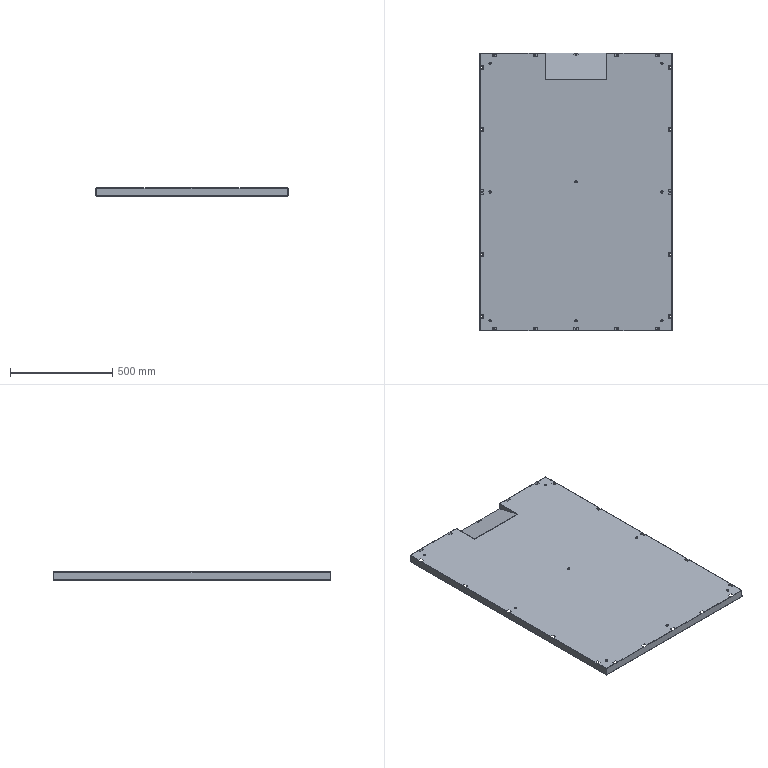Part | SolidWorks | 2 solids | 400 faces | box 939 x 1359 x 40 mm | volume 1511582 mm3 | plane 254 | cylinder 126 | spline 20 | commonest cylinder face diameters 7 x50 0.4 x30 2.4 x30 11 x16